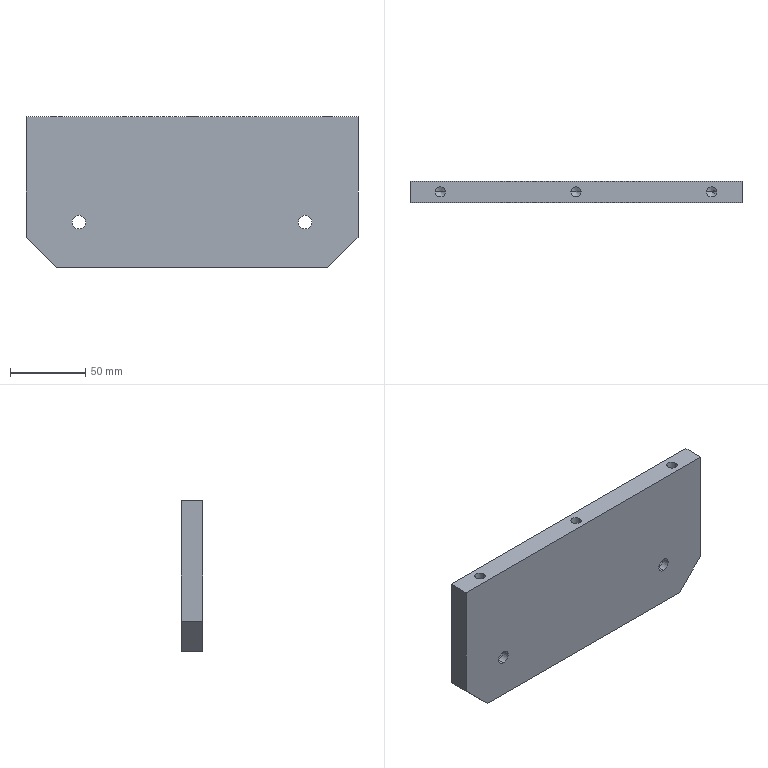Part | STEP file | fBY02F02M-00-05A | 1 solid | 30 faces | box 220 x 14 x 100 mm | volume 295677 mm3 | cylinder 14 | plane 10 | cone 6 | commonest cylinder face diameters 6.8 x6 9 x4 14 x4